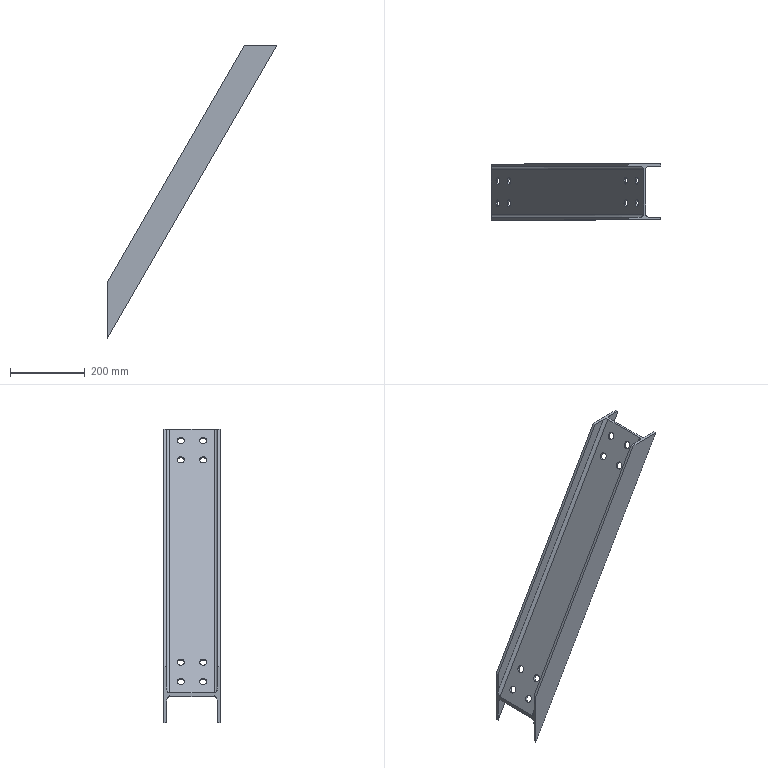Part | STEP file | Powder bin diagonal beam 5_Default<As Machined> | 1 solid | 34 faces | box 453.301 x 150 x 785.141 mm | volume 1452308 mm3 | cylinder 20 | plane 14 | commonest cylinder face diameters 19 x16 16 x4